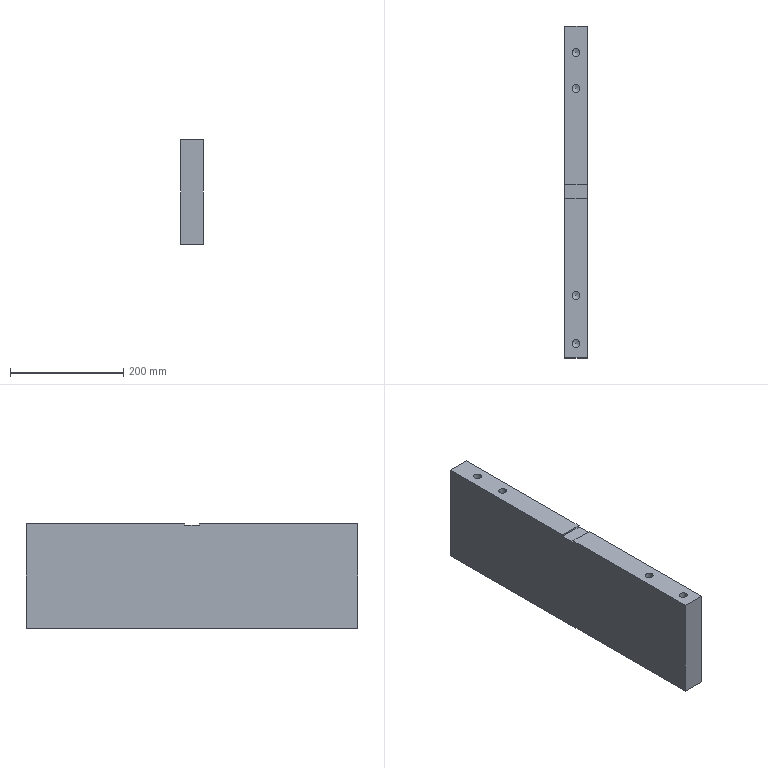Part | STEP file | 1 solid | 24 faces | box 40 x 585 x 185 mm | volume 4281820 mm3 | plane 10 | cylinder 7 | cone 7 | commonest cylinder face diameters 14 x7
STEP:
#1=CARTESIAN_POINT('',(25.,-12.5,-107.));
#2=VERTEX_POINT('',#1);
#3=CARTESIAN_POINT('',(65.,-12.5,-107.));
#4=VERTEX_POINT('',#3);
#5=CARTESIAN_POINT('',(483.5,-12.5,-107.));
#6=DIRECTION('',(1.,0.,0.));
#7=VECTOR('',#6,1.);
#8=LINE('',#5,#7);
#9=EDGE_CURVE('',#2,#4,#8,.T.);
#10=ORIENTED_EDGE('',*,*,#9,.F.);
#11=CARTESIAN_POINT('',(25.,-292.5,-107.));
#12=VERTEX_POINT('',#11);
#13=CARTESIAN_POINT('',(25.,-1.,-107.));
#14=DIRECTION('',(0.,-1.,0.));
#15=VECTOR('',#14,1.);
#16=LINE('',#13,#15);
#17=EDGE_CURVE('',#2,#12,#16,.T.);
#18=ORIENTED_EDGE('',*,*,#17,.T.);
#19=CARTESIAN_POINT('',(65.,-292.5,-107.));
#20=VERTEX_POINT('',#19);
#21=CARTESIAN_POINT('',(483.5,-292.5,-107.));
#22=DIRECTION('',(1.,0.,0.));
#23=VECTOR('',#22,1.);
#24=LINE('',#21,#23);
#25=EDGE_CURVE('',#12,#20,#24,.T.);
#26=ORIENTED_EDGE('',*,*,#25,.T.);
#27=CARTESIAN_POINT('',(65.,-1.,-107.));
#28=DIRECTION('',(0.,1.,0.));
#29=VECTOR('',#28,1.);
#30=LINE('',#27,#29);
#31=EDGE_CURVE('',#20,#4,#30,.T.);
#32=ORIENTED_EDGE('',*,*,#31,.T.);
#33=EDGE_LOOP('',(#10,#18,#26,#32));
#34=FACE_BOUND('',#33,.T.);
#35=CARTESIAN_POINT('',(38.,-267.5,-107.));
#36=VERTEX_POINT('',#35);
#37=CARTESIAN_POINT('',(45.,-267.5,-107.));
#38=DIRECTION('',(0.,0.,-1.));
#39=DIRECTION('',(-1.,0.,0.));
#40=AXIS2_PLACEMENT_3D('',#37,#38,#39);
#41=CIRCLE('',#40,7.);
#42=EDGE_CURVE('',#36,#36,#41,.T.);
#43=ORIENTED_EDGE('',*,*,#42,.T.);
#44=EDGE_LOOP('',(#43));
#45=FACE_BOUND('',#44,.T.);
#46=CARTESIAN_POINT('',(38.,-182.5,-107.));
#47=VERTEX_POINT('',#46);
#48=CARTESIAN_POINT('',(45.,-182.5,-107.));
#49=DIRECTION('',(0.,0.,-1.));
#50=DIRECTION('',(-1.,0.,0.));
#51=AXIS2_PLACEMENT_3D('',#48,#49,#50);
#52=CIRCLE('',#51,7.);
#53=EDGE_CURVE('',#47,#47,#52,.T.);
#54=ORIENTED_EDGE('',*,*,#53,.T.);
#55=EDGE_LOOP('',(#54));
#56=FACE_BOUND('',#55,.T.);
#57=CARTESIAN_POINT('',(483.5,-1.,-107.));
#58=DIRECTION('',(0.,0.,1.));
#59=DIRECTION('',(1.,0.,0.));
#60=AXIS2_PLACEMENT_3D('',#57,#58,#59);
#61=PLANE('',#60);
#62=ADVANCED_FACE('',(#34,#45,#56),#61,.T.);
#63=ORIENTED_EDGE('',*,*,#17,.F.);
#64=CARTESIAN_POINT('',(25.,-12.5,-110.));
#65=VERTEX_POINT('',#64);
#66=CARTESIAN_POINT('',(25.,-12.5,-107.));
#67=DIRECTION('',(0.,0.,-1.));
#68=VECTOR('',#67,1.);
#69=LINE('',#66,#68);
#70=EDGE_CURVE('',#2,#65,#69,.T.);
#71=ORIENTED_EDGE('',*,*,#70,.T.);
#72=CARTESIAN_POINT('',(25.,12.5,-110.));
#73=VERTEX_POINT('',#72);
#74=CARTESIAN_POINT('',(25.,-1.,-110.));
#75=DIRECTION('',(0.,1.,0.));
#76=VECTOR('',#75,1.);
#77=LINE('',#74,#76);
#78=EDGE_CURVE('',#65,#73,#77,.T.);
#79=ORIENTED_EDGE('',*,*,#78,.T.);
#80=CARTESIAN_POINT('',(25.,12.5,-107.));
#81=VERTEX_POINT('',#80);
#82=CARTESIAN_POINT('',(25.,12.5,-107.));
#83=DIRECTION('',(0.,0.,1.));
#84=VECTOR('',#83,1.);
#85=LINE('',#82,#84);
#86=EDGE_CURVE('',#73,#81,#85,.T.);
#87=ORIENTED_EDGE('',*,*,#86,.T.);
#88=CARTESIAN_POINT('',(25.,292.5,-107.));
#89=VERTEX_POINT('',#88);
#90=CARTESIAN_POINT('',(25.,-1.,-107.));
#91=DIRECTION('',(0.,-1.,0.));
#92=VECTOR('',#91,1.);
#93=LINE('',#90,#92);
#94=EDGE_CURVE('',#89,#81,#93,.T.);
#95=ORIENTED_EDGE('',*,*,#94,.F.);
#96=CARTESIAN_POINT('',(25.,292.5,-292.));
#97=VERTEX_POINT('',#96);
#98=CARTESIAN_POINT('',(25.,292.5,-107.));
#99=DIRECTION('',(0.,0.,1.));
#100=VECTOR('',#99,1.);
#101=LINE('',#98,#100);
#102=EDGE_CURVE('',#97,#89,#101,.T.);
#103=ORIENTED_EDGE('',*,*,#102,.F.);
#104=CARTESIAN_POINT('',(25.,-292.5,-292.));
#105=VERTEX_POINT('',#104);
#106=CARTESIAN_POINT('',(25.,-1.,-292.));
#107=DIRECTION('',(0.,-1.,0.));
#108=VECTOR('',#107,1.);
#109=LINE('',#106,#108);
#110=EDGE_CURVE('',#97,#105,#109,.T.);
#111=ORIENTED_EDGE('',*,*,#110,.T.);
#112=CARTESIAN_POINT('',(25.,-292.5,-107.));
#113=DIRECTION('',(0.,0.,1.));
#114=VECTOR('',#113,1.);
#115=LINE('',#112,#114);
#116=EDGE_CURVE('',#105,#12,#115,.T.);
#117=ORIENTED_EDGE('',*,*,#116,.T.);
#118=EDGE_LOOP('',(#63,#71,#79,#87,#95,#103,#111,#117));
#119=FACE_OUTER_BOUND('',#118,.T.);
#120=CARTESIAN_POINT('',(25.,-1.,-107.));
#121=DIRECTION('',(-1.,0.,0.));
#122=DIRECTION('',(0.,-1.,0.));
#123=AXIS2_PLACEMENT_3D('',#120,#121,#122);
#124=PLANE('',#123);
#125=ADVANCED_FACE('',(#119),#124,.T.);
#126=ORIENTED_EDGE('',*,*,#102,.T.);
#127=CARTESIAN_POINT('',(65.,292.5,-107.));
#128=VERTEX_POINT('',#127);
#129=CARTESIAN_POINT('',(483.5,292.5,-107.));
#130=DIRECTION('',(-1.,0.,0.));
#131=VECTOR('',#130,1.);
#132=LINE('',#129,#131);
#133=EDGE_CURVE('',#128,#89,#132,.T.);
#134=ORIENTED_EDGE('',*,*,#133,.F.);
#135=CARTESIAN_POINT('',(65.,292.5,-292.));
#136=VERTEX_POINT('',#135);
#137=CARTESIAN_POINT('',(65.,292.5,-107.));
#138=DIRECTION('',(0.,0.,1.));
#139=VECTOR('',#138,1.);
#140=LINE('',#137,#139);
#141=EDGE_CURVE('',#136,#128,#140,.T.);
#142=ORIENTED_EDGE('',*,*,#141,.F.);
#143=CARTESIAN_POINT('',(483.5,292.5,-292.));
#144=DIRECTION('',(-1.,0.,0.));
#145=VECTOR('',#144,1.);
#146=LINE('',#143,#145);
#147=EDGE_CURVE('',#136,#97,#146,.T.);
#148=ORIENTED_EDGE('',*,*,#147,.T.);
#149=EDGE_LOOP('',(#126,#134,#142,#148));
#150=FACE_OUTER_BOUND('',#149,.T.);
#151=CARTESIAN_POINT('',(483.5,292.5,-107.));
#152=DIRECTION('',(0.,1.,0.));
#153=DIRECTION('',(-1.,0.,0.));
#154=AXIS2_PLACEMENT_3D('',#151,#152,#153);
#155=PLANE('',#154);
#156=ADVANCED_FACE('',(#150),#155,.T.);
#157=CARTESIAN_POINT('',(65.,12.5,-110.));
#158=VERTEX_POINT('',#157);
#159=CARTESIAN_POINT('',(65.,-12.5,-110.));
#160=VERTEX_POINT('',#159);
#161=CARTESIAN_POINT('',(65.,-1.,-110.));
#162=DIRECTION('',(0.,-1.,0.));
#163=VECTOR('',#162,1.);
#164=LINE('',#161,#163);
#165=EDGE_CURVE('',#158,#160,#164,.T.);
#166=ORIENTED_EDGE('',*,*,#165,.T.);
#167=CARTESIAN_POINT('',(65.,-12.5,-107.));
#168=DIRECTION('',(0.,0.,1.));
#169=VECTOR('',#168,1.);
#170=LINE('',#167,#169);
#171=EDGE_CURVE('',#160,#4,#170,.T.);
#172=ORIENTED_EDGE('',*,*,#171,.T.);
#173=ORIENTED_EDGE('',*,*,#31,.F.);
#174=CARTESIAN_POINT('',(65.,-292.5,-292.));
#175=VERTEX_POINT('',#174);
#176=CARTESIAN_POINT('',(65.,-292.5,-107.));
#177=DIRECTION('',(0.,0.,1.));
#178=VECTOR('',#177,1.);
#179=LINE('',#176,#178);
#180=EDGE_CURVE('',#175,#20,#179,.T.);
#181=ORIENTED_EDGE('',*,*,#180,.F.);
#182=CARTESIAN_POINT('',(65.,-1.,-292.));
#183=DIRECTION('',(0.,1.,0.));
#184=VECTOR('',#183,1.);
#185=LINE('',#182,#184);
#186=EDGE_CURVE('',#175,#136,#185,.T.);
#187=ORIENTED_EDGE('',*,*,#186,.T.);
#188=ORIENTED_EDGE('',*,*,#141,.T.);
#189=CARTESIAN_POINT('',(65.,12.5,-107.));
#190=VERTEX_POINT('',#189);
#191=CARTESIAN_POINT('',(65.,-1.,-107.));
#192=DIRECTION('',(0.,1.,0.));
#193=VECTOR('',#192,1.);
#194=LINE('',#191,#193);
#195=EDGE_CURVE('',#190,#128,#194,.T.);
#196=ORIENTED_EDGE('',*,*,#195,.F.);
#197=CARTESIAN_POINT('',(65.,12.5,-107.));
#198=DIRECTION('',(0.,0.,-1.));
#199=VECTOR('',#198,1.);
#200=LINE('',#197,#199);
#201=EDGE_CURVE('',#190,#158,#200,.T.);
#202=ORIENTED_EDGE('',*,*,#201,.T.);
#203=EDGE_LOOP('',(#166,#172,#173,#181,#187,#188,#196,#202));
#204=FACE_OUTER_BOUND('',#203,.T.);
#205=CARTESIAN_POINT('',(65.,-1.,-107.));
#206=DIRECTION('',(1.,0.,0.));
#207=DIRECTION('',(0.,1.,0.));
#208=AXIS2_PLACEMENT_3D('',#205,#206,#207);
#209=PLANE('',#208);
#210=ADVANCED_FACE('',(#204),#209,.T.);
#211=CARTESIAN_POINT('',(483.5,-292.5,-292.));
#212=DIRECTION('',(1.,0.,0.));
#213=VECTOR('',#212,1.);
#214=LINE('',#211,#213);
#215=EDGE_CURVE('',#105,#175,#214,.T.);
#216=ORIENTED_EDGE('',*,*,#215,.T.);
#217=ORIENTED_EDGE('',*,*,#180,.T.);
#218=ORIENTED_EDGE('',*,*,#25,.F.);
#219=ORIENTED_EDGE('',*,*,#116,.F.);
#220=EDGE_LOOP('',(#216,#217,#218,#219));
#221=FACE_OUTER_BOUND('',#220,.T.);
#222=CARTESIAN_POINT('',(483.5,-292.5,-107.));
#223=DIRECTION('',(0.,-1.,0.));
#224=DIRECTION('',(1.,0.,0.));
#225=AXIS2_PLACEMENT_3D('',#222,#223,#224);
#226=PLANE('',#225);
#227=ADVANCED_FACE('',(#221),#226,.T.);
#228=CARTESIAN_POINT('',(483.5,12.5,-107.));
#229=DIRECTION('',(-1.,0.,0.));
#230=VECTOR('',#229,1.);
#231=LINE('',#228,#230);
#232=EDGE_CURVE('',#190,#81,#231,.T.);
#233=ORIENTED_EDGE('',*,*,#232,.F.);
#234=ORIENTED_EDGE('',*,*,#195,.T.);
#235=ORIENTED_EDGE('',*,*,#133,.T.);
#236=ORIENTED_EDGE('',*,*,#94,.T.);
#237=EDGE_LOOP('',(#233,#234,#235,#236));
#238=FACE_BOUND('',#237,.T.);
#239=CARTESIAN_POINT('',(38.,245.5,-107.));
#240=VERTEX_POINT('',#239);
#241=CARTESIAN_POINT('',(45.,245.5,-107.));
#242=DIRECTION('',(0.,0.,1.));
#243=DIRECTION('',(-1.,0.,0.));
#244=AXIS2_PLACEMENT_3D('',#241,#242,#243);
#245=CIRCLE('',#244,7.);
#246=EDGE_CURVE('',#240,#240,#245,.T.);
#247=ORIENTED_EDGE('',*,*,#246,.F.);
#248=EDGE_LOOP('',(#247));
#249=FACE_BOUND('',#248,.T.);
#250=CARTESIAN_POINT('',(38.,182.5,-107.));
#251=VERTEX_POINT('',#250);
#252=CARTESIAN_POINT('',(45.,182.5,-107.));
#253=DIRECTION('',(0.,0.,1.));
#254=DIRECTION('',(-1.,0.,0.));
#255=AXIS2_PLACEMENT_3D('',#252,#253,#254);
#256=CIRCLE('',#255,7.);
#257=EDGE_CURVE('',#251,#251,#256,.T.);
#258=ORIENTED_EDGE('',*,*,#257,.F.);
#259=EDGE_LOOP('',(#258));
#260=FACE_BOUND('',#259,.T.);
#261=CARTESIAN_POINT('',(483.5,-1.,-107.));
#262=DIRECTION('',(0.,0.,1.));
#263=DIRECTION('',(1.,0.,0.));
#264=AXIS2_PLACEMENT_3D('',#261,#262,#263);
#265=PLANE('',#264);
#266=ADVANCED_FACE('',(#238,#249,#260),#265,.T.);
#267=ORIENTED_EDGE('',*,*,#186,.F.);
#268=ORIENTED_EDGE('',*,*,#215,.F.);
#269=ORIENTED_EDGE('',*,*,#110,.F.);
#270=ORIENTED_EDGE('',*,*,#147,.F.);
#271=EDGE_LOOP('',(#267,#268,#269,#270));
#272=FACE_BOUND('',#271,.T.);
#273=CARTESIAN_POINT('',(52.,267.5,-292.));
#274=VERTEX_POINT('',#273);
#275=CARTESIAN_POINT('',(45.,267.5,-292.));
#276=DIRECTION('',(0.,0.,1.));
#277=DIRECTION('',(1.,0.,0.));
#278=AXIS2_PLACEMENT_3D('',#275,#276,#277);
#279=CIRCLE('',#278,7.);
#280=EDGE_CURVE('',#274,#274,#279,.T.);
#281=ORIENTED_EDGE('',*,*,#280,.T.);
#282=EDGE_LOOP('',(#281));
#283=FACE_BOUND('',#282,.T.);
#284=CARTESIAN_POINT('',(52.,-267.5,-292.));
#285=VERTEX_POINT('',#284);
#286=CARTESIAN_POINT('',(45.,-267.5,-292.));
#287=DIRECTION('',(0.,0.,-1.));
#288=DIRECTION('',(1.,0.,0.));
#289=AXIS2_PLACEMENT_3D('',#286,#287,#288);
#290=CIRCLE('',#289,7.);
#291=EDGE_CURVE('',#285,#285,#290,.T.);
#292=ORIENTED_EDGE('',*,*,#291,.F.);
#293=EDGE_LOOP('',(#292));
#294=FACE_BOUND('',#293,.T.);
#295=CARTESIAN_POINT('',(52.,0.,-292.));
#296=VERTEX_POINT('',#295);
#297=CARTESIAN_POINT('',(45.,0.,-292.));
#298=DIRECTION('',(0.,0.,1.));
#299=DIRECTION('',(1.,0.,0.));
#300=AXIS2_PLACEMENT_3D('',#297,#298,#299);
#301=CIRCLE('',#300,7.);
#302=EDGE_CURVE('',#296,#296,#301,.T.);
#303=ORIENTED_EDGE('',*,*,#302,.T.);
#304=EDGE_LOOP('',(#303));
#305=FACE_BOUND('',#304,.T.);
#306=CARTESIAN_POINT('',(473.5,-1.,-292.));
#307=DIRECTION('',(0.,0.,-1.));
#308=DIRECTION('',(1.,0.,0.));
#309=AXIS2_PLACEMENT_3D('',#306,#307,#308);
#310=PLANE('',#309);
#311=ADVANCED_FACE('',(#272,#283,#294,#305),#310,.T.);
#312=CARTESIAN_POINT('',(47.,-12.5,-110.));
#313=DIRECTION('',(-1.,0.,0.));
#314=VECTOR('',#313,1.);
#315=LINE('',#312,#314);
#316=EDGE_CURVE('',#160,#65,#315,.T.);
#317=ORIENTED_EDGE('',*,*,#316,.F.);
#318=ORIENTED_EDGE('',*,*,#165,.F.);
#319=CARTESIAN_POINT('',(47.,12.5,-110.));
#320=DIRECTION('',(1.,0.,0.));
#321=VECTOR('',#320,1.);
#322=LINE('',#319,#321);
#323=EDGE_CURVE('',#73,#158,#322,.T.);
#324=ORIENTED_EDGE('',*,*,#323,.F.);
#325=ORIENTED_EDGE('',*,*,#78,.F.);
#326=EDGE_LOOP('',(#317,#318,#324,#325));
#327=FACE_OUTER_BOUND('',#326,.T.);
#328=CARTESIAN_POINT('',(47.,0.,-110.));
#329=DIRECTION('',(0.,0.,-1.));
#330=DIRECTION('',(-1.,0.,0.));
#331=AXIS2_PLACEMENT_3D('',#328,#329,#330);
#332=PLANE('',#331);
#333=ADVANCED_FACE('',(#327),#332,.F.);
#334=ORIENTED_EDGE('',*,*,#9,.T.);
#335=ORIENTED_EDGE('',*,*,#171,.F.);
#336=ORIENTED_EDGE('',*,*,#316,.T.);
#337=ORIENTED_EDGE('',*,*,#70,.F.);
#338=EDGE_LOOP('',(#334,#335,#336,#337));
#339=FACE_OUTER_BOUND('',#338,.T.);
#340=CARTESIAN_POINT('',(47.,-12.5,-108.));
#341=DIRECTION('',(0.,-1.,0.));
#342=DIRECTION('',(0.,0.,-1.));
#343=AXIS2_PLACEMENT_3D('',#340,#341,#342);
#344=PLANE('',#343);
#345=ADVANCED_FACE('',(#339),#344,.F.);
#346=ORIENTED_EDGE('',*,*,#323,.T.);
#347=ORIENTED_EDGE('',*,*,#201,.F.);
#348=ORIENTED_EDGE('',*,*,#232,.T.);
#349=ORIENTED_EDGE('',*,*,#86,.F.);
#350=EDGE_LOOP('',(#346,#347,#348,#349));
#351=FACE_OUTER_BOUND('',#350,.T.);
#352=CARTESIAN_POINT('',(47.,12.5,-108.));
#353=DIRECTION('',(0.,1.,0.));
#354=DIRECTION('',(0.,0.,1.));
#355=AXIS2_PLACEMENT_3D('',#352,#353,#354);
#356=PLANE('',#355);
#357=ADVANCED_FACE('',(#351),#356,.F.);
#358=CARTESIAN_POINT('',(52.,-267.5,-147.));
#359=VERTEX_POINT('',#358);
#360=CARTESIAN_POINT('',(45.,-267.5,-147.));
#361=DIRECTION('',(0.,0.,1.));
#362=DIRECTION('',(1.,0.,0.));
#363=AXIS2_PLACEMENT_3D('',#360,#361,#362);
#364=CIRCLE('',#363,7.);
#365=EDGE_CURVE('',#359,#359,#364,.T.);
#366=ORIENTED_EDGE('',*,*,#365,.F.);
#367=EDGE_LOOP('',(#366));
#368=FACE_BOUND('',#367,.T.);
#369=ORIENTED_EDGE('',*,*,#42,.F.);
#370=EDGE_LOOP('',(#369));
#371=FACE_BOUND('',#370,.T.);
#372=CARTESIAN_POINT('',(45.,-267.5,-107.));
#373=DIRECTION('',(0.,0.,-1.));
#374=DIRECTION('',(1.,0.,0.));
#375=AXIS2_PLACEMENT_3D('',#372,#373,#374);
#376=CYLINDRICAL_SURFACE('',#375,7.);
#377=ADVANCED_FACE('',(#368,#371),#376,.F.);
#378=ORIENTED_EDGE('',*,*,#365,.T.);
#379=EDGE_LOOP('',(#378));
#380=FACE_BOUND('',#379,.T.);
#381=CARTESIAN_POINT('',(45.,-267.5,-150.));
#382=VERTEX_POINT('',#381);
#383=VERTEX_LOOP('',#382);
#384=FACE_BOUND('',#383,.T.);
#385=CARTESIAN_POINT('',(45.,-267.5,-150.));
#386=DIRECTION('',(0.,0.,1.));
#387=DIRECTION('',(1.,0.,0.));
#388=AXIS2_PLACEMENT_3D('',#385,#386,#387);
#389=CONICAL_SURFACE('',#388,0.,66.801);
#390=ADVANCED_FACE('',(#380,#384),#389,.F.);
#391=CARTESIAN_POINT('',(52.,245.5,-147.));
#392=VERTEX_POINT('',#391);
#393=CARTESIAN_POINT('',(45.,245.5,-147.));
#394=DIRECTION('',(0.,0.,-1.));
#395=DIRECTION('',(1.,0.,0.));
#396=AXIS2_PLACEMENT_3D('',#393,#394,#395);
#397=CIRCLE('',#396,7.);
#398=EDGE_CURVE('',#392,#392,#397,.T.);
#399=ORIENTED_EDGE('',*,*,#398,.T.);
#400=EDGE_LOOP('',(#399));
#401=FACE_BOUND('',#400,.T.);
#402=ORIENTED_EDGE('',*,*,#246,.T.);
#403=EDGE_LOOP('',(#402));
#404=FACE_BOUND('',#403,.T.);
#405=CARTESIAN_POINT('',(45.,245.5,-107.));
#406=DIRECTION('',(0.,0.,-1.));
#407=DIRECTION('',(1.,0.,0.));
#408=AXIS2_PLACEMENT_3D('',#405,#406,#407);
#409=CYLINDRICAL_SURFACE('',#408,7.);
#410=ADVANCED_FACE('',(#401,#404),#409,.F.);
#411=ORIENTED_EDGE('',*,*,#398,.F.);
#412=EDGE_LOOP('',(#411));
#413=FACE_BOUND('',#412,.T.);
#414=CARTESIAN_POINT('',(45.,245.5,-150.));
#415=VERTEX_POINT('',#414);
#416=VERTEX_LOOP('',#415);
#417=FACE_BOUND('',#416,.T.);
#418=CARTESIAN_POINT('',(45.,245.5,-150.));
#419=DIRECTION('',(0.,0.,1.));
#420=DIRECTION('',(1.,0.,0.));
#421=AXIS2_PLACEMENT_3D('',#418,#419,#420);
#422=CONICAL_SURFACE('',#421,0.,66.801);
#423=ADVANCED_FACE('',(#413,#417),#422,.F.);
#424=CARTESIAN_POINT('',(52.,-182.5,-147.));
#425=VERTEX_POINT('',#424);
#426=CARTESIAN_POINT('',(45.,-182.5,-147.));
#427=DIRECTION('',(0.,0.,1.));
#428=DIRECTION('',(1.,0.,0.));
#429=AXIS2_PLACEMENT_3D('',#426,#427,#428);
#430=CIRCLE('',#429,7.);
#431=EDGE_CURVE('',#425,#425,#430,.T.);
#432=ORIENTED_EDGE('',*,*,#431,.F.);
#433=EDGE_LOOP('',(#432));
#434=FACE_BOUND('',#433,.T.);
#435=ORIENTED_EDGE('',*,*,#53,.F.);
#436=EDGE_LOOP('',(#435));
#437=FACE_BOUND('',#436,.T.);
#438=CARTESIAN_POINT('',(45.,-182.5,-107.));
#439=DIRECTION('',(0.,0.,-1.));
#440=DIRECTION('',(1.,0.,0.));
#441=AXIS2_PLACEMENT_3D('',#438,#439,#440);
#442=CYLINDRICAL_SURFACE('',#441,7.);
#443=ADVANCED_FACE('',(#434,#437),#442,.F.);
#444=ORIENTED_EDGE('',*,*,#431,.T.);
#445=EDGE_LOOP('',(#444));
#446=FACE_BOUND('',#445,.T.);
#447=CARTESIAN_POINT('',(45.,-182.5,-150.));
#448=VERTEX_POINT('',#447);
#449=VERTEX_LOOP('',#448);
#450=FACE_BOUND('',#449,.T.);
#451=CARTESIAN_POINT('',(45.,-182.5,-150.));
#452=DIRECTION('',(0.,0.,1.));
#453=DIRECTION('',(1.,0.,0.));
#454=AXIS2_PLACEMENT_3D('',#451,#452,#453);
#455=CONICAL_SURFACE('',#454,0.,66.801);
#456=ADVANCED_FACE('',(#446,#450),#455,.F.);
#457=CARTESIAN_POINT('',(52.,182.5,-147.));
#458=VERTEX_POINT('',#457);
#459=CARTESIAN_POINT('',(45.,182.5,-147.));
#460=DIRECTION('',(0.,0.,-1.));
#461=DIRECTION('',(1.,0.,0.));
#462=AXIS2_PLACEMENT_3D('',#459,#460,#461);
#463=CIRCLE('',#462,7.);
#464=EDGE_CURVE('',#458,#458,#463,.T.);
#465=ORIENTED_EDGE('',*,*,#464,.T.);
#466=EDGE_LOOP('',(#465));
#467=FACE_BOUND('',#466,.T.);
#468=ORIENTED_EDGE('',*,*,#257,.T.);
#469=EDGE_LOOP('',(#468));
#470=FACE_BOUND('',#469,.T.);
#471=CARTESIAN_POINT('',(45.,182.5,-107.));
#472=DIRECTION('',(0.,0.,-1.));
#473=DIRECTION('',(1.,0.,0.));
#474=AXIS2_PLACEMENT_3D('',#471,#472,#473);
#475=CYLINDRICAL_SURFACE('',#474,7.);
#476=ADVANCED_FACE('',(#467,#470),#475,.F.);
#477=ORIENTED_EDGE('',*,*,#464,.F.);
#478=EDGE_LOOP('',(#477));
#479=FACE_BOUND('',#478,.T.);
#480=CARTESIAN_POINT('',(45.,182.5,-150.));
#481=VERTEX_POINT('',#480);
#482=VERTEX_LOOP('',#481);
#483=FACE_BOUND('',#482,.T.);
#484=CARTESIAN_POINT('',(45.,182.5,-150.));
#485=DIRECTION('',(0.,0.,1.));
#486=DIRECTION('',(1.,0.,0.));
#487=AXIS2_PLACEMENT_3D('',#484,#485,#486);
#488=CONICAL_SURFACE('',#487,0.,66.801);
#489=ADVANCED_FACE('',(#479,#483),#488,.F.);
#490=CARTESIAN_POINT('',(38.,267.5,-252.));
#491=VERTEX_POINT('',#490);
#492=CARTESIAN_POINT('',(45.,267.5,-252.));
#493=DIRECTION('',(0.,0.,-1.));
#494=DIRECTION('',(-1.,0.,0.));
#495=AXIS2_PLACEMENT_3D('',#492,#493,#494);
#496=CIRCLE('',#495,7.);
#497=EDGE_CURVE('',#491,#491,#496,.T.);
#498=ORIENTED_EDGE('',*,*,#497,.F.);
#499=EDGE_LOOP('',(#498));
#500=FACE_BOUND('',#499,.T.);
#501=ORIENTED_EDGE('',*,*,#280,.F.);
#502=EDGE_LOOP('',(#501));
#503=FACE_BOUND('',#502,.T.);
#504=CARTESIAN_POINT('',(45.,267.5,-292.));
#505=DIRECTION('',(0.,0.,1.));
#506=DIRECTION('',(-1.,0.,0.));
#507=AXIS2_PLACEMENT_3D('',#504,#505,#506);
#508=CYLINDRICAL_SURFACE('',#507,7.);
#509=ADVANCED_FACE('',(#500,#503),#508,.F.);
#510=ORIENTED_EDGE('',*,*,#497,.T.);
#511=EDGE_LOOP('',(#510));
#512=FACE_BOUND('',#511,.T.);
#513=CARTESIAN_POINT('',(45.,267.5,-249.));
#514=VERTEX_POINT('',#513);
#515=VERTEX_LOOP('',#514);
#516=FACE_BOUND('',#515,.T.);
#517=CARTESIAN_POINT('',(45.,267.5,-249.));
#518=DIRECTION('',(0.,0.,-1.));
#519=DIRECTION('',(-1.,0.,0.));
#520=AXIS2_PLACEMENT_3D('',#517,#518,#519);
#521=CONICAL_SURFACE('',#520,0.,66.801);
#522=ADVANCED_FACE('',(#512,#516),#521,.F.);
#523=CARTESIAN_POINT('',(38.,-267.5,-252.));
#524=VERTEX_POINT('',#523);
#525=CARTESIAN_POINT('',(45.,-267.5,-252.));
#526=DIRECTION('',(0.,0.,1.));
#527=DIRECTION('',(-1.,0.,0.));
#528=AXIS2_PLACEMENT_3D('',#525,#526,#527);
#529=CIRCLE('',#528,7.);
#530=EDGE_CURVE('',#524,#524,#529,.T.);
#531=ORIENTED_EDGE('',*,*,#530,.T.);
#532=EDGE_LOOP('',(#531));
#533=FACE_BOUND('',#532,.T.);
#534=ORIENTED_EDGE('',*,*,#291,.T.);
#535=EDGE_LOOP('',(#534));
#536=FACE_BOUND('',#535,.T.);
#537=CARTESIAN_POINT('',(45.,-267.5,-292.));
#538=DIRECTION('',(0.,0.,1.));
#539=DIRECTION('',(-1.,0.,0.));
#540=AXIS2_PLACEMENT_3D('',#537,#538,#539);
#541=CYLINDRICAL_SURFACE('',#540,7.);
#542=ADVANCED_FACE('',(#533,#536),#541,.F.);
#543=ORIENTED_EDGE('',*,*,#530,.F.);
#544=EDGE_LOOP('',(#543));
#545=FACE_BOUND('',#544,.T.);
#546=CARTESIAN_POINT('',(45.,-267.5,-249.));
#547=VERTEX_POINT('',#546);
#548=VERTEX_LOOP('',#547);
#549=FACE_BOUND('',#548,.T.);
#550=CARTESIAN_POINT('',(45.,-267.5,-249.));
#551=DIRECTION('',(0.,0.,-1.));
#552=DIRECTION('',(-1.,0.,0.));
#553=AXIS2_PLACEMENT_3D('',#550,#551,#552);
#554=CONICAL_SURFACE('',#553,0.,66.801);
#555=ADVANCED_FACE('',(#545,#549),#554,.F.);
#556=CARTESIAN_POINT('',(38.,0.,-252.));
#557=VERTEX_POINT('',#556);
#558=CARTESIAN_POINT('',(45.,0.,-252.));
#559=DIRECTION('',(0.,0.,-1.));
#560=DIRECTION('',(-1.,0.,0.));
#561=AXIS2_PLACEMENT_3D('',#558,#559,#560);
#562=CIRCLE('',#561,7.);
#563=EDGE_CURVE('',#557,#557,#562,.T.);
#564=ORIENTED_EDGE('',*,*,#563,.F.);
#565=EDGE_LOOP('',(#564));
#566=FACE_BOUND('',#565,.T.);
#567=ORIENTED_EDGE('',*,*,#302,.F.);
#568=EDGE_LOOP('',(#567));
#569=FACE_BOUND('',#568,.T.);
#570=CARTESIAN_POINT('',(45.,0.,-292.));
#571=DIRECTION('',(0.,0.,1.));
#572=DIRECTION('',(-1.,0.,0.));
#573=AXIS2_PLACEMENT_3D('',#570,#571,#572);
#574=CYLINDRICAL_SURFACE('',#573,7.);
#575=ADVANCED_FACE('',(#566,#569),#574,.F.);
#576=ORIENTED_EDGE('',*,*,#563,.T.);
#577=EDGE_LOOP('',(#576));
#578=FACE_BOUND('',#577,.T.);
#579=CARTESIAN_POINT('',(45.,0.,-249.));
#580=VERTEX_POINT('',#579);
#581=VERTEX_LOOP('',#580);
#582=FACE_BOUND('',#581,.T.);
#583=CARTESIAN_POINT('',(45.,0.,-249.));
#584=DIRECTION('',(0.,0.,-1.));
#585=DIRECTION('',(-1.,0.,0.));
#586=AXIS2_PLACEMENT_3D('',#583,#584,#585);
#587=CONICAL_SURFACE('',#586,0.,66.801);
#588=ADVANCED_FACE('',(#578,#582),#587,.F.);
#589=CLOSED_SHELL('',(#62,#125,#156,#210,#227,#266,#311,#333,#345,#357,#377,#390,#410,#423,#443,#456,#476,#489,#509,#522,#542,#555,#575,#588));
#590=MANIFOLD_SOLID_BREP('',#589);
#591=(LENGTH_UNIT()NAMED_UNIT(*)SI_UNIT(.MILLI.,.METRE.));
#592=UNCERTAINTY_MEASURE_WITH_UNIT(LENGTH_MEASURE(0.00002),#591,'','');
#593=(NAMED_UNIT(*)PLANE_ANGLE_UNIT()SI_UNIT($,.RADIAN.));
#594=PLANE_ANGLE_MEASURE_WITH_UNIT(PLANE_ANGLE_MEASURE(0.01745),#593);
#595=DIMENSIONAL_EXPONENTS(0.,0.,0.,0.,0.,0.,0.);
#596=(CONVERSION_BASED_UNIT('DEGREE',#594)NAMED_UNIT(#595)PLANE_ANGLE_UNIT());
#597=(NAMED_UNIT(*)SI_UNIT($,.STERADIAN.)SOLID_ANGLE_UNIT());
#598=(GEOMETRIC_REPRESENTATION_CONTEXT(3)GLOBAL_UNCERTAINTY_ASSIGNED_CONTEXT((#592))GLOBAL_UNIT_ASSIGNED_CONTEXT((#591,#596,#597))REPRESENTATION_CONTEXT('',''));
#599=ADVANCED_BREP_SHAPE_REPRESENTATION('',(#590),#598);